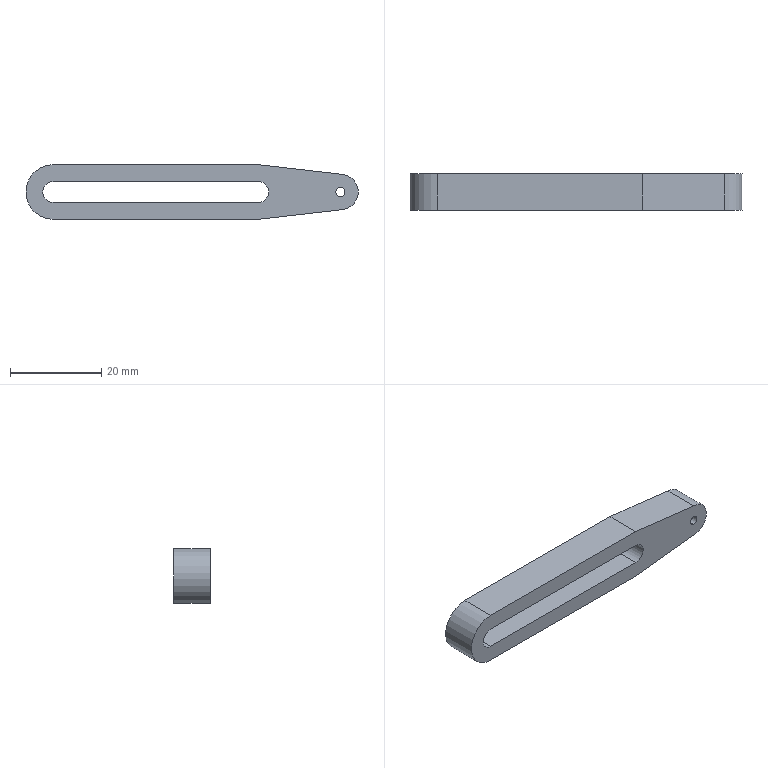Part | SolidWorks | features Cut 2, Extrusion 1 | 1 solid | 17 faces | box 72.914 x 8 x 12 mm | volume 4560 mm3 | plane 9 | cylinder 8 | commonest cylinder face diameters 2 x2 4 x2 4.6 x2 7.829 x1 12 x1
STEP:
#1=CARTESIAN_POINT('',(63.,6.,-1.));
#2=VERTEX_POINT('',#1);
#3=CARTESIAN_POINT('',(63.,6.,1.));
#4=VERTEX_POINT('',#3);
#5=CARTESIAN_POINT('',(63.,6.,0.));
#6=DIRECTION('',(0.,1.,0.));
#7=DIRECTION('',(0.,0.,1.));
#8=AXIS2_PLACEMENT_3D('',#5,#6,#7);
#9=CIRCLE('',#8,1.);
#10=EDGE_CURVE('',#2,#4,#9,.T.);
#11=ORIENTED_EDGE('',*,*,#10,.T.);
#12=CARTESIAN_POINT('',(63.,0.,1.));
#13=VERTEX_POINT('',#12);
#14=CARTESIAN_POINT('',(63.,8.,1.));
#15=DIRECTION('',(0.,-1.,0.));
#16=VECTOR('',#15,1000.);
#17=LINE('',#14,#16);
#18=EDGE_CURVE('',#4,#13,#17,.T.);
#19=ORIENTED_EDGE('',*,*,#18,.T.);
#20=CARTESIAN_POINT('',(63.,0.,-1.));
#21=VERTEX_POINT('',#20);
#22=CARTESIAN_POINT('',(63.,0.,0.));
#23=DIRECTION('',(0.,-1.,0.));
#24=DIRECTION('',(0.,0.,-1.));
#25=AXIS2_PLACEMENT_3D('',#22,#23,#24);
#26=CIRCLE('',#25,1.);
#27=EDGE_CURVE('',#13,#21,#26,.T.);
#28=ORIENTED_EDGE('',*,*,#27,.T.);
#29=CARTESIAN_POINT('',(63.,8.,-1.));
#30=DIRECTION('',(0.,-1.,0.));
#31=VECTOR('',#30,1000.);
#32=LINE('',#29,#31);
#33=EDGE_CURVE('',#2,#21,#32,.T.);
#34=ORIENTED_EDGE('',*,*,#33,.F.);
#35=EDGE_LOOP('',(#11,#19,#28,#34));
#36=FACE_OUTER_BOUND('',#35,.T.);
#37=CARTESIAN_POINT('',(63.,8.,0.));
#38=DIRECTION('',(0.,-1.,0.));
#39=DIRECTION('',(0.,0.,-1.));
#40=AXIS2_PLACEMENT_3D('',#37,#38,#39);
#41=CYLINDRICAL_SURFACE('',#40,1.);
#42=ADVANCED_FACE('',(#36),#41,.F.);
#43=CARTESIAN_POINT('',(63.,6.,-2.));
#44=VERTEX_POINT('',#43);
#45=CARTESIAN_POINT('',(63.,6.,2.));
#46=VERTEX_POINT('',#45);
#47=CARTESIAN_POINT('',(63.,6.,0.));
#48=DIRECTION('',(0.,1.,0.));
#49=DIRECTION('',(0.,0.,1.));
#50=AXIS2_PLACEMENT_3D('',#47,#48,#49);
#51=CIRCLE('',#50,2.);
#52=EDGE_CURVE('',#44,#46,#51,.T.);
#53=ORIENTED_EDGE('',*,*,#52,.F.);
#54=CARTESIAN_POINT('',(63.,8.,-2.));
#55=VERTEX_POINT('',#54);
#56=CARTESIAN_POINT('',(63.,6.,-2.));
#57=DIRECTION('',(0.,1.,0.));
#58=VECTOR('',#57,1000.);
#59=LINE('',#56,#58);
#60=EDGE_CURVE('',#44,#55,#59,.T.);
#61=ORIENTED_EDGE('',*,*,#60,.T.);
#62=CARTESIAN_POINT('',(63.,8.,2.));
#63=VERTEX_POINT('',#62);
#64=CARTESIAN_POINT('',(63.,8.,0.));
#65=DIRECTION('',(0.,1.,0.));
#66=DIRECTION('',(0.,0.,1.));
#67=AXIS2_PLACEMENT_3D('',#64,#65,#66);
#68=CIRCLE('',#67,2.);
#69=EDGE_CURVE('',#55,#63,#68,.T.);
#70=ORIENTED_EDGE('',*,*,#69,.T.);
#71=CARTESIAN_POINT('',(63.,6.,2.));
#72=DIRECTION('',(0.,1.,0.));
#73=VECTOR('',#72,1000.);
#74=LINE('',#71,#73);
#75=EDGE_CURVE('',#46,#63,#74,.T.);
#76=ORIENTED_EDGE('',*,*,#75,.F.);
#77=EDGE_LOOP('',(#53,#61,#70,#76));
#78=FACE_OUTER_BOUND('',#77,.T.);
#79=CARTESIAN_POINT('',(63.,6.,0.));
#80=DIRECTION('',(0.,1.,0.));
#81=DIRECTION('',(0.,0.,1.));
#82=AXIS2_PLACEMENT_3D('',#79,#80,#81);
#83=CYLINDRICAL_SURFACE('',#82,2.);
#84=ADVANCED_FACE('',(#78),#83,.F.);
#85=CARTESIAN_POINT('',(63.,8.,0.));
#86=DIRECTION('',(0.,1.,0.));
#87=DIRECTION('',(0.,0.,1.));
#88=AXIS2_PLACEMENT_3D('',#85,#86,#87);
#89=CIRCLE('',#88,2.);
#90=EDGE_CURVE('',#63,#55,#89,.T.);
#91=ORIENTED_EDGE('',*,*,#90,.F.);
#92=ORIENTED_EDGE('',*,*,#69,.F.);
#93=EDGE_LOOP('',(#91,#92));
#94=FACE_BOUND('',#93,.T.);
#95=CARTESIAN_POINT('',(0.,8.,-6.));
#96=VERTEX_POINT('',#95);
#97=CARTESIAN_POINT('',(0.,8.,6.));
#98=VERTEX_POINT('',#97);
#99=CARTESIAN_POINT('',(0.,8.,0.));
#100=DIRECTION('',(0.,1.,0.));
#101=DIRECTION('',(0.,0.,1.));
#102=AXIS2_PLACEMENT_3D('',#99,#100,#101);
#103=CIRCLE('',#102,6.);
#104=EDGE_CURVE('',#96,#98,#103,.T.);
#105=ORIENTED_EDGE('',*,*,#104,.T.);
#106=CARTESIAN_POINT('',(45.,8.,6.));
#107=VERTEX_POINT('',#106);
#108=CARTESIAN_POINT('',(0.,8.,6.));
#109=DIRECTION('',(1.,0.,0.));
#110=VECTOR('',#109,1000.);
#111=LINE('',#108,#110);
#112=EDGE_CURVE('',#98,#107,#111,.T.);
#113=ORIENTED_EDGE('',*,*,#112,.T.);
#114=CARTESIAN_POINT('',(63.,8.,3.914));
#115=VERTEX_POINT('',#114);
#116=CARTESIAN_POINT('',(45.,8.,6.));
#117=DIRECTION('',(0.9934,0.,-0.1151));
#118=VECTOR('',#117,1000.);
#119=LINE('',#116,#118);
#120=EDGE_CURVE('',#107,#115,#119,.T.);
#121=ORIENTED_EDGE('',*,*,#120,.T.);
#122=CARTESIAN_POINT('',(63.,8.,-3.914));
#123=VERTEX_POINT('',#122);
#124=CARTESIAN_POINT('',(63.,8.,0.));
#125=DIRECTION('',(0.,1.,0.));
#126=DIRECTION('',(0.,0.,1.));
#127=AXIS2_PLACEMENT_3D('',#124,#125,#126);
#128=CIRCLE('',#127,3.914);
#129=EDGE_CURVE('',#115,#123,#128,.T.);
#130=ORIENTED_EDGE('',*,*,#129,.T.);
#131=CARTESIAN_POINT('',(45.,8.,-6.));
#132=VERTEX_POINT('',#131);
#133=CARTESIAN_POINT('',(45.,8.,-6.));
#134=DIRECTION('',(-0.9934,0.,-0.1151));
#135=VECTOR('',#134,1000.);
#136=LINE('',#133,#135);
#137=EDGE_CURVE('',#123,#132,#136,.T.);
#138=ORIENTED_EDGE('',*,*,#137,.T.);
#139=CARTESIAN_POINT('',(0.,8.,-6.));
#140=DIRECTION('',(-1.,0.,0.));
#141=VECTOR('',#140,1000.);
#142=LINE('',#139,#141);
#143=EDGE_CURVE('',#132,#96,#142,.T.);
#144=ORIENTED_EDGE('',*,*,#143,.T.);
#145=EDGE_LOOP('',(#105,#113,#121,#130,#138,#144));
#146=FACE_OUTER_BOUND('',#145,.T.);
#147=CARTESIAN_POINT('',(0.,8.,2.3));
#148=VERTEX_POINT('',#147);
#149=CARTESIAN_POINT('',(45.,8.,2.3));
#150=VERTEX_POINT('',#149);
#151=CARTESIAN_POINT('',(0.,8.,2.3));
#152=DIRECTION('',(1.,0.,0.));
#153=VECTOR('',#152,1000.);
#154=LINE('',#151,#153);
#155=EDGE_CURVE('',#148,#150,#154,.T.);
#156=ORIENTED_EDGE('',*,*,#155,.F.);
#157=CARTESIAN_POINT('',(0.,8.,-2.3));
#158=VERTEX_POINT('',#157);
#159=CARTESIAN_POINT('',(0.,8.,0.));
#160=DIRECTION('',(0.,1.,0.));
#161=DIRECTION('',(0.,0.,1.));
#162=AXIS2_PLACEMENT_3D('',#159,#160,#161);
#163=CIRCLE('',#162,2.3);
#164=EDGE_CURVE('',#158,#148,#163,.T.);
#165=ORIENTED_EDGE('',*,*,#164,.F.);
#166=CARTESIAN_POINT('',(45.,8.,-2.3));
#167=VERTEX_POINT('',#166);
#168=CARTESIAN_POINT('',(0.,8.,-2.3));
#169=DIRECTION('',(-1.,0.,0.));
#170=VECTOR('',#169,1000.);
#171=LINE('',#168,#170);
#172=EDGE_CURVE('',#167,#158,#171,.T.);
#173=ORIENTED_EDGE('',*,*,#172,.F.);
#174=CARTESIAN_POINT('',(45.,8.,0.));
#175=DIRECTION('',(0.,1.,0.));
#176=DIRECTION('',(0.,0.,1.));
#177=AXIS2_PLACEMENT_3D('',#174,#175,#176);
#178=CIRCLE('',#177,2.3);
#179=EDGE_CURVE('',#150,#167,#178,.T.);
#180=ORIENTED_EDGE('',*,*,#179,.F.);
#181=EDGE_LOOP('',(#156,#165,#173,#180));
#182=FACE_BOUND('',#181,.T.);
#183=CARTESIAN_POINT('',(0.,8.,0.));
#184=DIRECTION('',(0.,1.,0.));
#185=DIRECTION('',(0.,0.,1.));
#186=AXIS2_PLACEMENT_3D('',#183,#184,#185);
#187=PLANE('',#186);
#188=ADVANCED_FACE('',(#94,#146,#182),#187,.T.);
#189=CARTESIAN_POINT('',(63.,0.,0.));
#190=DIRECTION('',(0.,-1.,0.));
#191=DIRECTION('',(0.,0.,-1.));
#192=AXIS2_PLACEMENT_3D('',#189,#190,#191);
#193=CIRCLE('',#192,1.);
#194=EDGE_CURVE('',#21,#13,#193,.T.);
#195=ORIENTED_EDGE('',*,*,#194,.F.);
#196=ORIENTED_EDGE('',*,*,#27,.F.);
#197=EDGE_LOOP('',(#195,#196));
#198=FACE_BOUND('',#197,.T.);
#199=CARTESIAN_POINT('',(0.,0.,-6.));
#200=VERTEX_POINT('',#199);
#201=CARTESIAN_POINT('',(0.,0.,6.));
#202=VERTEX_POINT('',#201);
#203=CARTESIAN_POINT('',(0.,0.,0.));
#204=DIRECTION('',(0.,1.,0.));
#205=DIRECTION('',(0.,0.,1.));
#206=AXIS2_PLACEMENT_3D('',#203,#204,#205);
#207=CIRCLE('',#206,6.);
#208=EDGE_CURVE('',#200,#202,#207,.T.);
#209=ORIENTED_EDGE('',*,*,#208,.F.);
#210=CARTESIAN_POINT('',(45.,0.,-6.));
#211=VERTEX_POINT('',#210);
#212=CARTESIAN_POINT('',(0.,0.,-6.));
#213=DIRECTION('',(-1.,0.,0.));
#214=VECTOR('',#213,1000.);
#215=LINE('',#212,#214);
#216=EDGE_CURVE('',#211,#200,#215,.T.);
#217=ORIENTED_EDGE('',*,*,#216,.F.);
#218=CARTESIAN_POINT('',(63.,0.,-3.914));
#219=VERTEX_POINT('',#218);
#220=CARTESIAN_POINT('',(45.,0.,-6.));
#221=DIRECTION('',(-0.9934,0.,-0.1151));
#222=VECTOR('',#221,1000.);
#223=LINE('',#220,#222);
#224=EDGE_CURVE('',#219,#211,#223,.T.);
#225=ORIENTED_EDGE('',*,*,#224,.F.);
#226=CARTESIAN_POINT('',(63.,0.,3.914));
#227=VERTEX_POINT('',#226);
#228=CARTESIAN_POINT('',(63.,0.,0.));
#229=DIRECTION('',(0.,1.,0.));
#230=DIRECTION('',(0.,0.,1.));
#231=AXIS2_PLACEMENT_3D('',#228,#229,#230);
#232=CIRCLE('',#231,3.914);
#233=EDGE_CURVE('',#227,#219,#232,.T.);
#234=ORIENTED_EDGE('',*,*,#233,.F.);
#235=CARTESIAN_POINT('',(45.,0.,6.));
#236=VERTEX_POINT('',#235);
#237=CARTESIAN_POINT('',(45.,0.,6.));
#238=DIRECTION('',(0.9934,0.,-0.1151));
#239=VECTOR('',#238,1000.);
#240=LINE('',#237,#239);
#241=EDGE_CURVE('',#236,#227,#240,.T.);
#242=ORIENTED_EDGE('',*,*,#241,.F.);
#243=CARTESIAN_POINT('',(0.,0.,6.));
#244=DIRECTION('',(1.,0.,0.));
#245=VECTOR('',#244,1000.);
#246=LINE('',#243,#245);
#247=EDGE_CURVE('',#202,#236,#246,.T.);
#248=ORIENTED_EDGE('',*,*,#247,.F.);
#249=EDGE_LOOP('',(#209,#217,#225,#234,#242,#248));
#250=FACE_OUTER_BOUND('',#249,.T.);
#251=CARTESIAN_POINT('',(0.,0.,-2.3));
#252=VERTEX_POINT('',#251);
#253=CARTESIAN_POINT('',(0.,0.,2.3));
#254=VERTEX_POINT('',#253);
#255=CARTESIAN_POINT('',(0.,0.,0.));
#256=DIRECTION('',(0.,1.,0.));
#257=DIRECTION('',(0.,0.,1.));
#258=AXIS2_PLACEMENT_3D('',#255,#256,#257);
#259=CIRCLE('',#258,2.3);
#260=EDGE_CURVE('',#252,#254,#259,.T.);
#261=ORIENTED_EDGE('',*,*,#260,.T.);
#262=CARTESIAN_POINT('',(45.,0.,2.3));
#263=VERTEX_POINT('',#262);
#264=CARTESIAN_POINT('',(0.,0.,2.3));
#265=DIRECTION('',(1.,0.,0.));
#266=VECTOR('',#265,1000.);
#267=LINE('',#264,#266);
#268=EDGE_CURVE('',#254,#263,#267,.T.);
#269=ORIENTED_EDGE('',*,*,#268,.T.);
#270=CARTESIAN_POINT('',(45.,0.,-2.3));
#271=VERTEX_POINT('',#270);
#272=CARTESIAN_POINT('',(45.,0.,0.));
#273=DIRECTION('',(0.,1.,0.));
#274=DIRECTION('',(0.,0.,1.));
#275=AXIS2_PLACEMENT_3D('',#272,#273,#274);
#276=CIRCLE('',#275,2.3);
#277=EDGE_CURVE('',#263,#271,#276,.T.);
#278=ORIENTED_EDGE('',*,*,#277,.T.);
#279=CARTESIAN_POINT('',(0.,0.,-2.3));
#280=DIRECTION('',(-1.,0.,0.));
#281=VECTOR('',#280,1000.);
#282=LINE('',#279,#281);
#283=EDGE_CURVE('',#271,#252,#282,.T.);
#284=ORIENTED_EDGE('',*,*,#283,.T.);
#285=EDGE_LOOP('',(#261,#269,#278,#284));
#286=FACE_BOUND('',#285,.T.);
#287=CARTESIAN_POINT('',(0.,0.,0.));
#288=DIRECTION('',(0.,1.,0.));
#289=DIRECTION('',(0.,0.,1.));
#290=AXIS2_PLACEMENT_3D('',#287,#288,#289);
#291=PLANE('',#290);
#292=ADVANCED_FACE('',(#198,#250,#286),#291,.F.);
#293=ORIENTED_EDGE('',*,*,#208,.T.);
#294=CARTESIAN_POINT('',(0.,8.,6.));
#295=DIRECTION('',(0.,-1.,0.));
#296=VECTOR('',#295,1000.);
#297=LINE('',#294,#296);
#298=EDGE_CURVE('',#98,#202,#297,.T.);
#299=ORIENTED_EDGE('',*,*,#298,.F.);
#300=ORIENTED_EDGE('',*,*,#104,.F.);
#301=CARTESIAN_POINT('',(0.,8.,-6.));
#302=DIRECTION('',(0.,-1.,0.));
#303=VECTOR('',#302,1000.);
#304=LINE('',#301,#303);
#305=EDGE_CURVE('',#96,#200,#304,.T.);
#306=ORIENTED_EDGE('',*,*,#305,.T.);
#307=EDGE_LOOP('',(#293,#299,#300,#306));
#308=FACE_OUTER_BOUND('',#307,.T.);
#309=CARTESIAN_POINT('',(0.,8.,0.));
#310=DIRECTION('',(0.,-1.,0.));
#311=DIRECTION('',(0.,0.,-1.));
#312=AXIS2_PLACEMENT_3D('',#309,#310,#311);
#313=CYLINDRICAL_SURFACE('',#312,6.);
#314=ADVANCED_FACE('',(#308),#313,.T.);
#315=ORIENTED_EDGE('',*,*,#247,.T.);
#316=CARTESIAN_POINT('',(45.,8.,6.));
#317=DIRECTION('',(0.,-1.,0.));
#318=VECTOR('',#317,1000.);
#319=LINE('',#316,#318);
#320=EDGE_CURVE('',#107,#236,#319,.T.);
#321=ORIENTED_EDGE('',*,*,#320,.F.);
#322=ORIENTED_EDGE('',*,*,#112,.F.);
#323=ORIENTED_EDGE('',*,*,#298,.T.);
#324=EDGE_LOOP('',(#315,#321,#322,#323));
#325=FACE_OUTER_BOUND('',#324,.T.);
#326=CARTESIAN_POINT('',(0.,8.,6.));
#327=DIRECTION('',(0.,0.,-1.));
#328=DIRECTION('',(-1.,0.,0.));
#329=AXIS2_PLACEMENT_3D('',#326,#327,#328);
#330=PLANE('',#329);
#331=ADVANCED_FACE('',(#325),#330,.F.);
#332=ORIENTED_EDGE('',*,*,#241,.T.);
#333=CARTESIAN_POINT('',(63.,8.,3.914));
#334=DIRECTION('',(0.,-1.,0.));
#335=VECTOR('',#334,1000.);
#336=LINE('',#333,#335);
#337=EDGE_CURVE('',#115,#227,#336,.T.);
#338=ORIENTED_EDGE('',*,*,#337,.F.);
#339=ORIENTED_EDGE('',*,*,#120,.F.);
#340=ORIENTED_EDGE('',*,*,#320,.T.);
#341=EDGE_LOOP('',(#332,#338,#339,#340));
#342=FACE_OUTER_BOUND('',#341,.T.);
#343=CARTESIAN_POINT('',(45.,8.,6.));
#344=DIRECTION('',(-0.1151,0.,-0.9934));
#345=DIRECTION('',(-0.9934,0.,0.1151));
#346=AXIS2_PLACEMENT_3D('',#343,#344,#345);
#347=PLANE('',#346);
#348=ADVANCED_FACE('',(#342),#347,.F.);
#349=ORIENTED_EDGE('',*,*,#233,.T.);
#350=CARTESIAN_POINT('',(63.,8.,-3.914));
#351=DIRECTION('',(0.,-1.,0.));
#352=VECTOR('',#351,1000.);
#353=LINE('',#350,#352);
#354=EDGE_CURVE('',#123,#219,#353,.T.);
#355=ORIENTED_EDGE('',*,*,#354,.F.);
#356=ORIENTED_EDGE('',*,*,#129,.F.);
#357=ORIENTED_EDGE('',*,*,#337,.T.);
#358=EDGE_LOOP('',(#349,#355,#356,#357));
#359=FACE_OUTER_BOUND('',#358,.T.);
#360=CARTESIAN_POINT('',(63.,8.,0.));
#361=DIRECTION('',(0.,-1.,0.));
#362=DIRECTION('',(0.,0.,-1.));
#363=AXIS2_PLACEMENT_3D('',#360,#361,#362);
#364=CYLINDRICAL_SURFACE('',#363,3.914);
#365=ADVANCED_FACE('',(#359),#364,.T.);
#366=ORIENTED_EDGE('',*,*,#224,.T.);
#367=CARTESIAN_POINT('',(45.,8.,-6.));
#368=DIRECTION('',(0.,-1.,0.));
#369=VECTOR('',#368,1000.);
#370=LINE('',#367,#369);
#371=EDGE_CURVE('',#132,#211,#370,.T.);
#372=ORIENTED_EDGE('',*,*,#371,.F.);
#373=ORIENTED_EDGE('',*,*,#137,.F.);
#374=ORIENTED_EDGE('',*,*,#354,.T.);
#375=EDGE_LOOP('',(#366,#372,#373,#374));
#376=FACE_OUTER_BOUND('',#375,.T.);
#377=CARTESIAN_POINT('',(45.,8.,-6.));
#378=DIRECTION('',(-0.1151,0.,0.9934));
#379=DIRECTION('',(0.9934,0.,0.1151));
#380=AXIS2_PLACEMENT_3D('',#377,#378,#379);
#381=PLANE('',#380);
#382=ADVANCED_FACE('',(#376),#381,.F.);
#383=ORIENTED_EDGE('',*,*,#216,.T.);
#384=ORIENTED_EDGE('',*,*,#305,.F.);
#385=ORIENTED_EDGE('',*,*,#143,.F.);
#386=ORIENTED_EDGE('',*,*,#371,.T.);
#387=EDGE_LOOP('',(#383,#384,#385,#386));
#388=FACE_OUTER_BOUND('',#387,.T.);
#389=CARTESIAN_POINT('',(0.,8.,-6.));
#390=DIRECTION('',(0.,0.,1.));
#391=DIRECTION('',(1.,0.,0.));
#392=AXIS2_PLACEMENT_3D('',#389,#390,#391);
#393=PLANE('',#392);
#394=ADVANCED_FACE('',(#388),#393,.F.);
#395=ORIENTED_EDGE('',*,*,#260,.F.);
#396=CARTESIAN_POINT('',(0.,8.,-2.3));
#397=DIRECTION('',(0.,-1.,0.));
#398=VECTOR('',#397,1000.);
#399=LINE('',#396,#398);
#400=EDGE_CURVE('',#158,#252,#399,.T.);
#401=ORIENTED_EDGE('',*,*,#400,.F.);
#402=ORIENTED_EDGE('',*,*,#164,.T.);
#403=CARTESIAN_POINT('',(0.,8.,2.3));
#404=DIRECTION('',(0.,-1.,0.));
#405=VECTOR('',#404,1000.);
#406=LINE('',#403,#405);
#407=EDGE_CURVE('',#148,#254,#406,.T.);
#408=ORIENTED_EDGE('',*,*,#407,.T.);
#409=EDGE_LOOP('',(#395,#401,#402,#408));
#410=FACE_OUTER_BOUND('',#409,.T.);
#411=CARTESIAN_POINT('',(0.,8.,0.));
#412=DIRECTION('',(0.,-1.,0.));
#413=DIRECTION('',(0.,0.,-1.));
#414=AXIS2_PLACEMENT_3D('',#411,#412,#413);
#415=CYLINDRICAL_SURFACE('',#414,2.3);
#416=ADVANCED_FACE('',(#410),#415,.F.);
#417=ORIENTED_EDGE('',*,*,#268,.F.);
#418=ORIENTED_EDGE('',*,*,#407,.F.);
#419=ORIENTED_EDGE('',*,*,#155,.T.);
#420=CARTESIAN_POINT('',(45.,8.,2.3));
#421=DIRECTION('',(0.,-1.,0.));
#422=VECTOR('',#421,1000.);
#423=LINE('',#420,#422);
#424=EDGE_CURVE('',#150,#263,#423,.T.);
#425=ORIENTED_EDGE('',*,*,#424,.T.);
#426=EDGE_LOOP('',(#417,#418,#419,#425));
#427=FACE_OUTER_BOUND('',#426,.T.);
#428=CARTESIAN_POINT('',(0.,8.,2.3));
#429=DIRECTION('',(0.,0.,-1.));
#430=DIRECTION('',(-1.,0.,0.));
#431=AXIS2_PLACEMENT_3D('',#428,#429,#430);
#432=PLANE('',#431);
#433=ADVANCED_FACE('',(#427),#432,.T.);
#434=ORIENTED_EDGE('',*,*,#277,.F.);
#435=ORIENTED_EDGE('',*,*,#424,.F.);
#436=ORIENTED_EDGE('',*,*,#179,.T.);
#437=CARTESIAN_POINT('',(45.,8.,-2.3));
#438=DIRECTION('',(0.,-1.,0.));
#439=VECTOR('',#438,1000.);
#440=LINE('',#437,#439);
#441=EDGE_CURVE('',#167,#271,#440,.T.);
#442=ORIENTED_EDGE('',*,*,#441,.T.);
#443=EDGE_LOOP('',(#434,#435,#436,#442));
#444=FACE_OUTER_BOUND('',#443,.T.);
#445=CARTESIAN_POINT('',(45.,8.,0.));
#446=DIRECTION('',(0.,-1.,0.));
#447=DIRECTION('',(0.,0.,-1.));
#448=AXIS2_PLACEMENT_3D('',#445,#446,#447);
#449=CYLINDRICAL_SURFACE('',#448,2.3);
#450=ADVANCED_FACE('',(#444),#449,.F.);
#451=ORIENTED_EDGE('',*,*,#283,.F.);
#452=ORIENTED_EDGE('',*,*,#441,.F.);
#453=ORIENTED_EDGE('',*,*,#172,.T.);
#454=ORIENTED_EDGE('',*,*,#400,.T.);
#455=EDGE_LOOP('',(#451,#452,#453,#454));
#456=FACE_OUTER_BOUND('',#455,.T.);
#457=CARTESIAN_POINT('',(0.,8.,-2.3));
#458=DIRECTION('',(0.,0.,1.));
#459=DIRECTION('',(1.,0.,0.));
#460=AXIS2_PLACEMENT_3D('',#457,#458,#459);
#461=PLANE('',#460);
#462=ADVANCED_FACE('',(#456),#461,.T.);
#463=ORIENTED_EDGE('',*,*,#60,.F.);
#464=CARTESIAN_POINT('',(63.,6.,0.));
#465=DIRECTION('',(0.,1.,0.));
#466=DIRECTION('',(0.,0.,1.));
#467=AXIS2_PLACEMENT_3D('',#464,#465,#466);
#468=CIRCLE('',#467,2.);
#469=EDGE_CURVE('',#46,#44,#468,.T.);
#470=ORIENTED_EDGE('',*,*,#469,.F.);
#471=ORIENTED_EDGE('',*,*,#75,.T.);
#472=ORIENTED_EDGE('',*,*,#90,.T.);
#473=EDGE_LOOP('',(#463,#470,#471,#472));
#474=FACE_OUTER_BOUND('',#473,.T.);
#475=CARTESIAN_POINT('',(63.,6.,0.));
#476=DIRECTION('',(0.,1.,0.));
#477=DIRECTION('',(0.,0.,1.));
#478=AXIS2_PLACEMENT_3D('',#475,#476,#477);
#479=CYLINDRICAL_SURFACE('',#478,2.);
#480=ADVANCED_FACE('',(#474),#479,.F.);
#481=ORIENTED_EDGE('',*,*,#10,.F.);
#482=CARTESIAN_POINT('',(63.,6.,0.));
#483=DIRECTION('',(0.,1.,0.));
#484=DIRECTION('',(0.,0.,1.));
#485=AXIS2_PLACEMENT_3D('',#482,#483,#484);
#486=CIRCLE('',#485,1.);
#487=EDGE_CURVE('',#4,#2,#486,.T.);
#488=ORIENTED_EDGE('',*,*,#487,.F.);
#489=EDGE_LOOP('',(#481,#488));
#490=FACE_BOUND('',#489,.T.);
#491=ORIENTED_EDGE('',*,*,#469,.T.);
#492=ORIENTED_EDGE('',*,*,#52,.T.);
#493=EDGE_LOOP('',(#491,#492));
#494=FACE_OUTER_BOUND('',#493,.T.);
#495=CARTESIAN_POINT('',(63.,6.,0.));
#496=DIRECTION('',(0.,1.,0.));
#497=DIRECTION('',(0.,0.,1.));
#498=AXIS2_PLACEMENT_3D('',#495,#496,#497);
#499=PLANE('',#498);
#500=ADVANCED_FACE('',(#490,#494),#499,.T.);
#501=ORIENTED_EDGE('',*,*,#18,.F.);
#502=ORIENTED_EDGE('',*,*,#487,.T.);
#503=ORIENTED_EDGE('',*,*,#33,.T.);
#504=ORIENTED_EDGE('',*,*,#194,.T.);
#505=EDGE_LOOP('',(#501,#502,#503,#504));
#506=FACE_OUTER_BOUND('',#505,.T.);
#507=CARTESIAN_POINT('',(63.,8.,0.));
#508=DIRECTION('',(0.,-1.,0.));
#509=DIRECTION('',(0.,0.,-1.));
#510=AXIS2_PLACEMENT_3D('',#507,#508,#509);
#511=CYLINDRICAL_SURFACE('',#510,1.);
#512=ADVANCED_FACE('',(#506),#511,.F.);
#513=CLOSED_SHELL('',(#42,#84,#188,#292,#314,#331,#348,#365,#382,#394,#416,#433,#450,#462,#480,#500,#512));
#514=MANIFOLD_SOLID_BREP('',#513);
#515=CARTESIAN_POINT('',(0.,0.,0.));
#516=DIRECTION('',(0.,0.,1.));
#517=DIRECTION('',(1.,0.,0.));
#518=AXIS2_PLACEMENT_3D('',#515,#516,#517);
#519=(LENGTH_UNIT()NAMED_UNIT(*)SI_UNIT(.MILLI.,.METRE.));
#520=UNCERTAINTY_MEASURE_WITH_UNIT(LENGTH_MEASURE(0.00001),#519,'','');
#521=(NAMED_UNIT(*)PLANE_ANGLE_UNIT()SI_UNIT($,.RADIAN.));
#522=(NAMED_UNIT(*)SI_UNIT($,.STERADIAN.)SOLID_ANGLE_UNIT());
#523=(GEOMETRIC_REPRESENTATION_CONTEXT(3)GLOBAL_UNCERTAINTY_ASSIGNED_CONTEXT((#520))GLOBAL_UNIT_ASSIGNED_CONTEXT((#519,#521,#522))REPRESENTATION_CONTEXT('',''));
#524=ADVANCED_BREP_SHAPE_REPRESENTATION('',(#514,#518),#523);